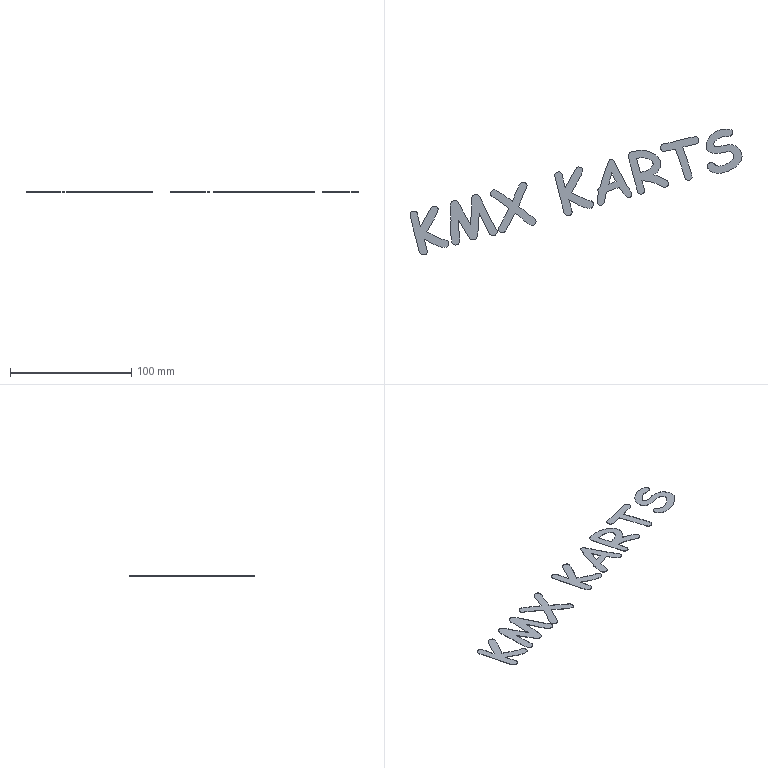Part | STEP file | KMX KART text | 8 solids | 214 faces | box 273.592 x 103.676 x 0.2 mm | volume 837.062 mm3 | spline 189 | plane 25